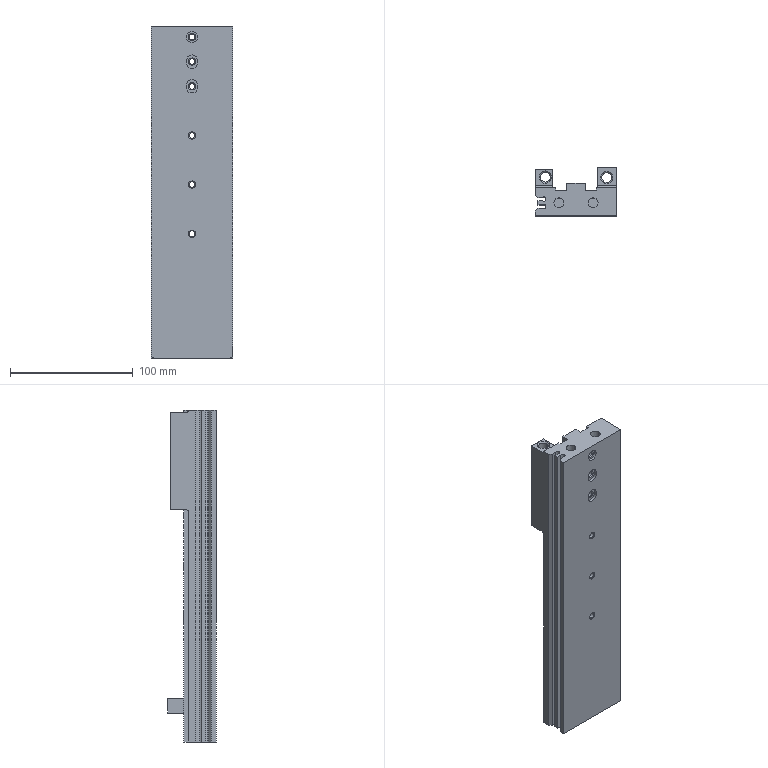Part | STEP file | 1 solid | 162 faces | box 66 x 39.5 x 270 mm | volume 335701 mm3 | cylinder 66 | plane 51 | cone 45 | commonest cylinder face diameters 4 x16 4.8 x12 10 x10 8 x8 9 x8 3.6 x4